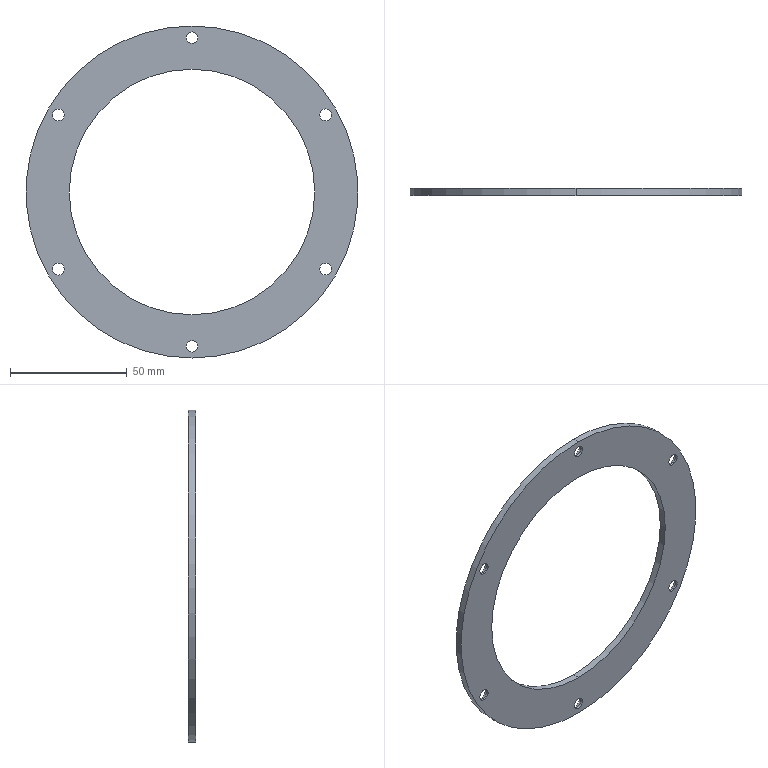Part | SolidWorks | features BaseBody 1 | 1 solid | 36 faces | box 142 x 3 x 142 mm | volume 20812 mm3 | cylinder 28 | plane 8 | commonest cylinder face diameters 5 x12 8 x12 105 x2 142 x2
STEP:
#1=CARTESIAN_POINT('',(0.,3.,52.5));
#2=VERTEX_POINT('',#1);
#3=CARTESIAN_POINT('',(0.,3.,-52.5));
#4=VERTEX_POINT('',#3);
#5=CARTESIAN_POINT('',(0.,3.,0.));
#6=DIRECTION('',(0.,-1.,0.));
#7=DIRECTION('',(0.,0.,-1.));
#8=AXIS2_PLACEMENT_3D('',#5,#6,#7);
#9=CIRCLE('',#8,52.5);
#10=EDGE_CURVE('',#2,#4,#9,.T.);
#11=ORIENTED_EDGE('',*,*,#10,.F.);
#12=CARTESIAN_POINT('',(0.,0.,52.5));
#13=VERTEX_POINT('',#12);
#14=CARTESIAN_POINT('',(0.,3.,52.5));
#15=DIRECTION('',(0.,-1.,0.));
#16=VECTOR('',#15,1000.);
#17=LINE('',#14,#16);
#18=EDGE_CURVE('',#2,#13,#17,.T.);
#19=ORIENTED_EDGE('',*,*,#18,.T.);
#20=CARTESIAN_POINT('',(0.,0.,-52.5));
#21=VERTEX_POINT('',#20);
#22=CARTESIAN_POINT('',(0.,0.,0.));
#23=DIRECTION('',(0.,-1.,0.));
#24=DIRECTION('',(0.,0.,-1.));
#25=AXIS2_PLACEMENT_3D('',#22,#23,#24);
#26=CIRCLE('',#25,52.5);
#27=EDGE_CURVE('',#13,#21,#26,.T.);
#28=ORIENTED_EDGE('',*,*,#27,.T.);
#29=CARTESIAN_POINT('',(0.,3.,-52.5));
#30=DIRECTION('',(0.,-1.,0.));
#31=VECTOR('',#30,1000.);
#32=LINE('',#29,#31);
#33=EDGE_CURVE('',#4,#21,#32,.T.);
#34=ORIENTED_EDGE('',*,*,#33,.F.);
#35=EDGE_LOOP('',(#11,#19,#28,#34));
#36=FACE_OUTER_BOUND('',#35,.T.);
#37=CARTESIAN_POINT('',(0.,3.,0.));
#38=DIRECTION('',(0.,-1.,0.));
#39=DIRECTION('',(0.,0.,-1.));
#40=AXIS2_PLACEMENT_3D('',#37,#38,#39);
#41=CYLINDRICAL_SURFACE('',#40,52.5);
#42=ADVANCED_FACE('',(#36),#41,.F.);
#43=CARTESIAN_POINT('',(0.,3.,-71.));
#44=VERTEX_POINT('',#43);
#45=CARTESIAN_POINT('',(0.,3.,71.));
#46=VERTEX_POINT('',#45);
#47=CARTESIAN_POINT('',(0.,3.,0.));
#48=DIRECTION('',(0.,-1.,0.));
#49=DIRECTION('',(0.,0.,-1.));
#50=AXIS2_PLACEMENT_3D('',#47,#48,#49);
#51=CIRCLE('',#50,71.);
#52=EDGE_CURVE('',#44,#46,#51,.T.);
#53=ORIENTED_EDGE('',*,*,#52,.T.);
#54=CARTESIAN_POINT('',(0.,0.,71.));
#55=VERTEX_POINT('',#54);
#56=CARTESIAN_POINT('',(0.,3.,71.));
#57=DIRECTION('',(0.,-1.,0.));
#58=VECTOR('',#57,1000.);
#59=LINE('',#56,#58);
#60=EDGE_CURVE('',#46,#55,#59,.T.);
#61=ORIENTED_EDGE('',*,*,#60,.T.);
#62=CARTESIAN_POINT('',(0.,0.,-71.));
#63=VERTEX_POINT('',#62);
#64=CARTESIAN_POINT('',(0.,0.,0.));
#65=DIRECTION('',(0.,1.,0.));
#66=DIRECTION('',(0.,0.,-1.));
#67=AXIS2_PLACEMENT_3D('',#64,#65,#66);
#68=CIRCLE('',#67,71.);
#69=EDGE_CURVE('',#55,#63,#68,.T.);
#70=ORIENTED_EDGE('',*,*,#69,.T.);
#71=CARTESIAN_POINT('',(0.,3.,-71.));
#72=DIRECTION('',(0.,-1.,0.));
#73=VECTOR('',#72,1000.);
#74=LINE('',#71,#73);
#75=EDGE_CURVE('',#44,#63,#74,.T.);
#76=ORIENTED_EDGE('',*,*,#75,.F.);
#77=EDGE_LOOP('',(#53,#61,#70,#76));
#78=FACE_OUTER_BOUND('',#77,.T.);
#79=CARTESIAN_POINT('',(0.,3.,0.));
#80=DIRECTION('',(0.,-1.,0.));
#81=DIRECTION('',(0.,0.,-1.));
#82=AXIS2_PLACEMENT_3D('',#79,#80,#81);
#83=CYLINDRICAL_SURFACE('',#82,71.);
#84=ADVANCED_FACE('',(#78),#83,.T.);
#85=CARTESIAN_POINT('',(0.,1.,68.5));
#86=VERTEX_POINT('',#85);
#87=CARTESIAN_POINT('',(0.,1.,63.5));
#88=VERTEX_POINT('',#87);
#89=CARTESIAN_POINT('',(0.,1.,66.));
#90=DIRECTION('',(0.,-1.,0.));
#91=DIRECTION('',(0.,0.,-1.));
#92=AXIS2_PLACEMENT_3D('',#89,#90,#91);
#93=CIRCLE('',#92,2.5);
#94=EDGE_CURVE('',#86,#88,#93,.T.);
#95=ORIENTED_EDGE('',*,*,#94,.F.);
#96=CARTESIAN_POINT('',(0.,0.,68.5));
#97=VERTEX_POINT('',#96);
#98=CARTESIAN_POINT('',(0.,3.,68.5));
#99=DIRECTION('',(0.,-1.,0.));
#100=VECTOR('',#99,1000.);
#101=LINE('',#98,#100);
#102=EDGE_CURVE('',#86,#97,#101,.T.);
#103=ORIENTED_EDGE('',*,*,#102,.T.);
#104=CARTESIAN_POINT('',(0.,0.,63.5));
#105=VERTEX_POINT('',#104);
#106=CARTESIAN_POINT('',(0.,0.,66.));
#107=DIRECTION('',(0.,-1.,0.));
#108=DIRECTION('',(0.,0.,-1.));
#109=AXIS2_PLACEMENT_3D('',#106,#107,#108);
#110=CIRCLE('',#109,2.5);
#111=EDGE_CURVE('',#97,#105,#110,.T.);
#112=ORIENTED_EDGE('',*,*,#111,.T.);
#113=CARTESIAN_POINT('',(0.,3.,63.5));
#114=DIRECTION('',(0.,-1.,0.));
#115=VECTOR('',#114,1000.);
#116=LINE('',#113,#115);
#117=EDGE_CURVE('',#88,#105,#116,.T.);
#118=ORIENTED_EDGE('',*,*,#117,.F.);
#119=EDGE_LOOP('',(#95,#103,#112,#118));
#120=FACE_OUTER_BOUND('',#119,.T.);
#121=CARTESIAN_POINT('',(0.,3.,66.));
#122=DIRECTION('',(0.,-1.,0.));
#123=DIRECTION('',(0.,0.,-1.));
#124=AXIS2_PLACEMENT_3D('',#121,#122,#123);
#125=CYLINDRICAL_SURFACE('',#124,2.5);
#126=ADVANCED_FACE('',(#120),#125,.F.);
#127=CARTESIAN_POINT('',(-57.158,1.,35.5));
#128=VERTEX_POINT('',#127);
#129=CARTESIAN_POINT('',(-57.158,1.,30.5));
#130=VERTEX_POINT('',#129);
#131=CARTESIAN_POINT('',(-57.158,1.,33.));
#132=DIRECTION('',(0.,-1.,0.));
#133=DIRECTION('',(0.,0.,-1.));
#134=AXIS2_PLACEMENT_3D('',#131,#132,#133);
#135=CIRCLE('',#134,2.5);
#136=EDGE_CURVE('',#128,#130,#135,.T.);
#137=ORIENTED_EDGE('',*,*,#136,.F.);
#138=CARTESIAN_POINT('',(-57.158,0.,35.5));
#139=VERTEX_POINT('',#138);
#140=CARTESIAN_POINT('',(-57.158,3.,35.5));
#141=DIRECTION('',(0.,-1.,0.));
#142=VECTOR('',#141,1000.);
#143=LINE('',#140,#142);
#144=EDGE_CURVE('',#128,#139,#143,.T.);
#145=ORIENTED_EDGE('',*,*,#144,.T.);
#146=CARTESIAN_POINT('',(-57.158,0.,30.5));
#147=VERTEX_POINT('',#146);
#148=CARTESIAN_POINT('',(-57.158,0.,33.));
#149=DIRECTION('',(0.,-1.,0.));
#150=DIRECTION('',(0.,0.,-1.));
#151=AXIS2_PLACEMENT_3D('',#148,#149,#150);
#152=CIRCLE('',#151,2.5);
#153=EDGE_CURVE('',#139,#147,#152,.T.);
#154=ORIENTED_EDGE('',*,*,#153,.T.);
#155=CARTESIAN_POINT('',(-57.158,3.,30.5));
#156=DIRECTION('',(0.,-1.,0.));
#157=VECTOR('',#156,1000.);
#158=LINE('',#155,#157);
#159=EDGE_CURVE('',#130,#147,#158,.T.);
#160=ORIENTED_EDGE('',*,*,#159,.F.);
#161=EDGE_LOOP('',(#137,#145,#154,#160));
#162=FACE_OUTER_BOUND('',#161,.T.);
#163=CARTESIAN_POINT('',(-57.158,3.,33.));
#164=DIRECTION('',(0.,-1.,0.));
#165=DIRECTION('',(0.,0.,-1.));
#166=AXIS2_PLACEMENT_3D('',#163,#164,#165);
#167=CYLINDRICAL_SURFACE('',#166,2.5);
#168=ADVANCED_FACE('',(#162),#167,.F.);
#169=CARTESIAN_POINT('',(-57.158,1.,-30.5));
#170=VERTEX_POINT('',#169);
#171=CARTESIAN_POINT('',(-57.158,1.,-35.5));
#172=VERTEX_POINT('',#171);
#173=CARTESIAN_POINT('',(-57.158,1.,-33.));
#174=DIRECTION('',(0.,-1.,0.));
#175=DIRECTION('',(0.,0.,-1.));
#176=AXIS2_PLACEMENT_3D('',#173,#174,#175);
#177=CIRCLE('',#176,2.5);
#178=EDGE_CURVE('',#170,#172,#177,.T.);
#179=ORIENTED_EDGE('',*,*,#178,.F.);
#180=CARTESIAN_POINT('',(-57.158,0.,-30.5));
#181=VERTEX_POINT('',#180);
#182=CARTESIAN_POINT('',(-57.158,3.,-30.5));
#183=DIRECTION('',(0.,-1.,0.));
#184=VECTOR('',#183,1000.);
#185=LINE('',#182,#184);
#186=EDGE_CURVE('',#170,#181,#185,.T.);
#187=ORIENTED_EDGE('',*,*,#186,.T.);
#188=CARTESIAN_POINT('',(-57.158,0.,-35.5));
#189=VERTEX_POINT('',#188);
#190=CARTESIAN_POINT('',(-57.158,0.,-33.));
#191=DIRECTION('',(0.,-1.,0.));
#192=DIRECTION('',(0.,0.,-1.));
#193=AXIS2_PLACEMENT_3D('',#190,#191,#192);
#194=CIRCLE('',#193,2.5);
#195=EDGE_CURVE('',#181,#189,#194,.T.);
#196=ORIENTED_EDGE('',*,*,#195,.T.);
#197=CARTESIAN_POINT('',(-57.158,3.,-35.5));
#198=DIRECTION('',(0.,-1.,0.));
#199=VECTOR('',#198,1000.);
#200=LINE('',#197,#199);
#201=EDGE_CURVE('',#172,#189,#200,.T.);
#202=ORIENTED_EDGE('',*,*,#201,.F.);
#203=EDGE_LOOP('',(#179,#187,#196,#202));
#204=FACE_OUTER_BOUND('',#203,.T.);
#205=CARTESIAN_POINT('',(-57.158,3.,-33.));
#206=DIRECTION('',(0.,-1.,0.));
#207=DIRECTION('',(0.,0.,-1.));
#208=AXIS2_PLACEMENT_3D('',#205,#206,#207);
#209=CYLINDRICAL_SURFACE('',#208,2.5);
#210=ADVANCED_FACE('',(#204),#209,.F.);
#211=CARTESIAN_POINT('',(0.,1.,-63.5));
#212=VERTEX_POINT('',#211);
#213=CARTESIAN_POINT('',(0.,1.,-68.5));
#214=VERTEX_POINT('',#213);
#215=CARTESIAN_POINT('',(0.,1.,-66.));
#216=DIRECTION('',(0.,-1.,0.));
#217=DIRECTION('',(0.,0.,-1.));
#218=AXIS2_PLACEMENT_3D('',#215,#216,#217);
#219=CIRCLE('',#218,2.5);
#220=EDGE_CURVE('',#212,#214,#219,.T.);
#221=ORIENTED_EDGE('',*,*,#220,.F.);
#222=CARTESIAN_POINT('',(0.,0.,-63.5));
#223=VERTEX_POINT('',#222);
#224=CARTESIAN_POINT('',(0.,3.,-63.5));
#225=DIRECTION('',(0.,-1.,0.));
#226=VECTOR('',#225,1000.);
#227=LINE('',#224,#226);
#228=EDGE_CURVE('',#212,#223,#227,.T.);
#229=ORIENTED_EDGE('',*,*,#228,.T.);
#230=CARTESIAN_POINT('',(0.,0.,-68.5));
#231=VERTEX_POINT('',#230);
#232=CARTESIAN_POINT('',(0.,0.,-66.));
#233=DIRECTION('',(0.,-1.,0.));
#234=DIRECTION('',(0.,0.,-1.));
#235=AXIS2_PLACEMENT_3D('',#232,#233,#234);
#236=CIRCLE('',#235,2.5);
#237=EDGE_CURVE('',#223,#231,#236,.T.);
#238=ORIENTED_EDGE('',*,*,#237,.T.);
#239=CARTESIAN_POINT('',(0.,3.,-68.5));
#240=DIRECTION('',(0.,-1.,0.));
#241=VECTOR('',#240,1000.);
#242=LINE('',#239,#241);
#243=EDGE_CURVE('',#214,#231,#242,.T.);
#244=ORIENTED_EDGE('',*,*,#243,.F.);
#245=EDGE_LOOP('',(#221,#229,#238,#244));
#246=FACE_OUTER_BOUND('',#245,.T.);
#247=CARTESIAN_POINT('',(0.,3.,-66.));
#248=DIRECTION('',(0.,-1.,0.));
#249=DIRECTION('',(0.,0.,-1.));
#250=AXIS2_PLACEMENT_3D('',#247,#248,#249);
#251=CYLINDRICAL_SURFACE('',#250,2.5);
#252=ADVANCED_FACE('',(#246),#251,.F.);
#253=CARTESIAN_POINT('',(57.158,1.,-30.5));
#254=VERTEX_POINT('',#253);
#255=CARTESIAN_POINT('',(57.158,1.,-35.5));
#256=VERTEX_POINT('',#255);
#257=CARTESIAN_POINT('',(57.158,1.,-33.));
#258=DIRECTION('',(0.,-1.,0.));
#259=DIRECTION('',(0.,0.,-1.));
#260=AXIS2_PLACEMENT_3D('',#257,#258,#259);
#261=CIRCLE('',#260,2.5);
#262=EDGE_CURVE('',#254,#256,#261,.T.);
#263=ORIENTED_EDGE('',*,*,#262,.F.);
#264=CARTESIAN_POINT('',(57.158,0.,-30.5));
#265=VERTEX_POINT('',#264);
#266=CARTESIAN_POINT('',(57.158,3.,-30.5));
#267=DIRECTION('',(0.,-1.,0.));
#268=VECTOR('',#267,1000.);
#269=LINE('',#266,#268);
#270=EDGE_CURVE('',#254,#265,#269,.T.);
#271=ORIENTED_EDGE('',*,*,#270,.T.);
#272=CARTESIAN_POINT('',(57.158,0.,-35.5));
#273=VERTEX_POINT('',#272);
#274=CARTESIAN_POINT('',(57.158,0.,-33.));
#275=DIRECTION('',(0.,-1.,0.));
#276=DIRECTION('',(0.,0.,-1.));
#277=AXIS2_PLACEMENT_3D('',#274,#275,#276);
#278=CIRCLE('',#277,2.5);
#279=EDGE_CURVE('',#265,#273,#278,.T.);
#280=ORIENTED_EDGE('',*,*,#279,.T.);
#281=CARTESIAN_POINT('',(57.158,3.,-35.5));
#282=DIRECTION('',(0.,-1.,0.));
#283=VECTOR('',#282,1000.);
#284=LINE('',#281,#283);
#285=EDGE_CURVE('',#256,#273,#284,.T.);
#286=ORIENTED_EDGE('',*,*,#285,.F.);
#287=EDGE_LOOP('',(#263,#271,#280,#286));
#288=FACE_OUTER_BOUND('',#287,.T.);
#289=CARTESIAN_POINT('',(57.158,3.,-33.));
#290=DIRECTION('',(0.,-1.,0.));
#291=DIRECTION('',(0.,0.,-1.));
#292=AXIS2_PLACEMENT_3D('',#289,#290,#291);
#293=CYLINDRICAL_SURFACE('',#292,2.5);
#294=ADVANCED_FACE('',(#288),#293,.F.);
#295=CARTESIAN_POINT('',(57.158,1.,35.5));
#296=VERTEX_POINT('',#295);
#297=CARTESIAN_POINT('',(57.158,1.,30.5));
#298=VERTEX_POINT('',#297);
#299=CARTESIAN_POINT('',(57.158,1.,33.));
#300=DIRECTION('',(0.,-1.,0.));
#301=DIRECTION('',(0.,0.,-1.));
#302=AXIS2_PLACEMENT_3D('',#299,#300,#301);
#303=CIRCLE('',#302,2.5);
#304=EDGE_CURVE('',#296,#298,#303,.T.);
#305=ORIENTED_EDGE('',*,*,#304,.F.);
#306=CARTESIAN_POINT('',(57.158,0.,35.5));
#307=VERTEX_POINT('',#306);
#308=CARTESIAN_POINT('',(57.158,3.,35.5));
#309=DIRECTION('',(0.,-1.,0.));
#310=VECTOR('',#309,1000.);
#311=LINE('',#308,#310);
#312=EDGE_CURVE('',#296,#307,#311,.T.);
#313=ORIENTED_EDGE('',*,*,#312,.T.);
#314=CARTESIAN_POINT('',(57.158,0.,30.5));
#315=VERTEX_POINT('',#314);
#316=CARTESIAN_POINT('',(57.158,0.,33.));
#317=DIRECTION('',(0.,-1.,0.));
#318=DIRECTION('',(0.,0.,-1.));
#319=AXIS2_PLACEMENT_3D('',#316,#317,#318);
#320=CIRCLE('',#319,2.5);
#321=EDGE_CURVE('',#307,#315,#320,.T.);
#322=ORIENTED_EDGE('',*,*,#321,.T.);
#323=CARTESIAN_POINT('',(57.158,3.,30.5));
#324=DIRECTION('',(0.,-1.,0.));
#325=VECTOR('',#324,1000.);
#326=LINE('',#323,#325);
#327=EDGE_CURVE('',#298,#315,#326,.T.);
#328=ORIENTED_EDGE('',*,*,#327,.F.);
#329=EDGE_LOOP('',(#305,#313,#322,#328));
#330=FACE_OUTER_BOUND('',#329,.T.);
#331=CARTESIAN_POINT('',(57.158,3.,33.));
#332=DIRECTION('',(0.,-1.,0.));
#333=DIRECTION('',(0.,0.,-1.));
#334=AXIS2_PLACEMENT_3D('',#331,#332,#333);
#335=CYLINDRICAL_SURFACE('',#334,2.5);
#336=ADVANCED_FACE('',(#330),#335,.F.);
#337=CARTESIAN_POINT('',(0.,1.,-70.));
#338=VERTEX_POINT('',#337);
#339=CARTESIAN_POINT('',(0.,1.,-62.));
#340=VERTEX_POINT('',#339);
#341=CARTESIAN_POINT('',(0.,1.,-66.));
#342=DIRECTION('',(0.,1.,0.));
#343=DIRECTION('',(0.,0.,1.));
#344=AXIS2_PLACEMENT_3D('',#341,#342,#343);
#345=CIRCLE('',#344,4.);
#346=EDGE_CURVE('',#338,#340,#345,.T.);
#347=ORIENTED_EDGE('',*,*,#346,.F.);
#348=CARTESIAN_POINT('',(0.,3.,-70.));
#349=VERTEX_POINT('',#348);
#350=CARTESIAN_POINT('',(0.,1.,-70.));
#351=DIRECTION('',(0.,1.,0.));
#352=VECTOR('',#351,1000.);
#353=LINE('',#350,#352);
#354=EDGE_CURVE('',#338,#349,#353,.T.);
#355=ORIENTED_EDGE('',*,*,#354,.T.);
#356=CARTESIAN_POINT('',(0.,3.,-62.));
#357=VERTEX_POINT('',#356);
#358=CARTESIAN_POINT('',(0.,3.,-66.));
#359=DIRECTION('',(0.,-1.,0.));
#360=DIRECTION('',(0.,0.,1.));
#361=AXIS2_PLACEMENT_3D('',#358,#359,#360);
#362=CIRCLE('',#361,4.);
#363=EDGE_CURVE('',#357,#349,#362,.T.);
#364=ORIENTED_EDGE('',*,*,#363,.F.);
#365=CARTESIAN_POINT('',(0.,1.,-62.));
#366=DIRECTION('',(0.,1.,0.));
#367=VECTOR('',#366,1000.);
#368=LINE('',#365,#367);
#369=EDGE_CURVE('',#340,#357,#368,.T.);
#370=ORIENTED_EDGE('',*,*,#369,.F.);
#371=EDGE_LOOP('',(#347,#355,#364,#370));
#372=FACE_OUTER_BOUND('',#371,.T.);
#373=CARTESIAN_POINT('',(0.,1.,-66.));
#374=DIRECTION('',(0.,1.,0.));
#375=DIRECTION('',(0.,0.,1.));
#376=AXIS2_PLACEMENT_3D('',#373,#374,#375);
#377=CYLINDRICAL_SURFACE('',#376,4.);
#378=ADVANCED_FACE('',(#372),#377,.F.);
#379=CARTESIAN_POINT('',(57.158,1.,-37.));
#380=VERTEX_POINT('',#379);
#381=CARTESIAN_POINT('',(57.158,1.,-29.));
#382=VERTEX_POINT('',#381);
#383=CARTESIAN_POINT('',(57.158,1.,-33.));
#384=DIRECTION('',(0.,1.,0.));
#385=DIRECTION('',(0.,0.,1.));
#386=AXIS2_PLACEMENT_3D('',#383,#384,#385);
#387=CIRCLE('',#386,4.);
#388=EDGE_CURVE('',#380,#382,#387,.T.);
#389=ORIENTED_EDGE('',*,*,#388,.F.);
#390=CARTESIAN_POINT('',(57.158,3.,-37.));
#391=VERTEX_POINT('',#390);
#392=CARTESIAN_POINT('',(57.158,1.,-37.));
#393=DIRECTION('',(0.,1.,0.));
#394=VECTOR('',#393,1000.);
#395=LINE('',#392,#394);
#396=EDGE_CURVE('',#380,#391,#395,.T.);
#397=ORIENTED_EDGE('',*,*,#396,.T.);
#398=CARTESIAN_POINT('',(57.158,3.,-29.));
#399=VERTEX_POINT('',#398);
#400=CARTESIAN_POINT('',(57.158,3.,-33.));
#401=DIRECTION('',(0.,-1.,0.));
#402=DIRECTION('',(0.,0.,1.));
#403=AXIS2_PLACEMENT_3D('',#400,#401,#402);
#404=CIRCLE('',#403,4.);
#405=EDGE_CURVE('',#399,#391,#404,.T.);
#406=ORIENTED_EDGE('',*,*,#405,.F.);
#407=CARTESIAN_POINT('',(57.158,1.,-29.));
#408=DIRECTION('',(0.,1.,0.));
#409=VECTOR('',#408,1000.);
#410=LINE('',#407,#409);
#411=EDGE_CURVE('',#382,#399,#410,.T.);
#412=ORIENTED_EDGE('',*,*,#411,.F.);
#413=EDGE_LOOP('',(#389,#397,#406,#412));
#414=FACE_OUTER_BOUND('',#413,.T.);
#415=CARTESIAN_POINT('',(57.158,1.,-33.));
#416=DIRECTION('',(0.,1.,0.));
#417=DIRECTION('',(0.,0.,1.));
#418=AXIS2_PLACEMENT_3D('',#415,#416,#417);
#419=CYLINDRICAL_SURFACE('',#418,4.);
#420=ADVANCED_FACE('',(#414),#419,.F.);
#421=CARTESIAN_POINT('',(57.158,1.,29.));
#422=VERTEX_POINT('',#421);
#423=CARTESIAN_POINT('',(57.158,1.,37.));
#424=VERTEX_POINT('',#423);
#425=CARTESIAN_POINT('',(57.158,1.,33.));
#426=DIRECTION('',(0.,1.,0.));
#427=DIRECTION('',(0.,0.,1.));
#428=AXIS2_PLACEMENT_3D('',#425,#426,#427);
#429=CIRCLE('',#428,4.);
#430=EDGE_CURVE('',#422,#424,#429,.T.);
#431=ORIENTED_EDGE('',*,*,#430,.F.);
#432=CARTESIAN_POINT('',(57.158,3.,29.));
#433=VERTEX_POINT('',#432);
#434=CARTESIAN_POINT('',(57.158,1.,29.));
#435=DIRECTION('',(0.,1.,0.));
#436=VECTOR('',#435,1000.);
#437=LINE('',#434,#436);
#438=EDGE_CURVE('',#422,#433,#437,.T.);
#439=ORIENTED_EDGE('',*,*,#438,.T.);
#440=CARTESIAN_POINT('',(57.158,3.,37.));
#441=VERTEX_POINT('',#440);
#442=CARTESIAN_POINT('',(57.158,3.,33.));
#443=DIRECTION('',(0.,-1.,0.));
#444=DIRECTION('',(0.,0.,1.));
#445=AXIS2_PLACEMENT_3D('',#442,#443,#444);
#446=CIRCLE('',#445,4.);
#447=EDGE_CURVE('',#441,#433,#446,.T.);
#448=ORIENTED_EDGE('',*,*,#447,.F.);
#449=CARTESIAN_POINT('',(57.158,1.,37.));
#450=DIRECTION('',(0.,1.,0.));
#451=VECTOR('',#450,1000.);
#452=LINE('',#449,#451);
#453=EDGE_CURVE('',#424,#441,#452,.T.);
#454=ORIENTED_EDGE('',*,*,#453,.F.);
#455=EDGE_LOOP('',(#431,#439,#448,#454));
#456=FACE_OUTER_BOUND('',#455,.T.);
#457=CARTESIAN_POINT('',(57.158,1.,33.));
#458=DIRECTION('',(0.,1.,0.));
#459=DIRECTION('',(0.,0.,1.));
#460=AXIS2_PLACEMENT_3D('',#457,#458,#459);
#461=CYLINDRICAL_SURFACE('',#460,4.);
#462=ADVANCED_FACE('',(#456),#461,.F.);
#463=CARTESIAN_POINT('',(0.,1.,62.));
#464=VERTEX_POINT('',#463);
#465=CARTESIAN_POINT('',(0.,1.,70.));
#466=VERTEX_POINT('',#465);
#467=CARTESIAN_POINT('',(0.,1.,66.));
#468=DIRECTION('',(0.,1.,0.));
#469=DIRECTION('',(0.,0.,1.));
#470=AXIS2_PLACEMENT_3D('',#467,#468,#469);
#471=CIRCLE('',#470,4.);
#472=EDGE_CURVE('',#464,#466,#471,.T.);
#473=ORIENTED_EDGE('',*,*,#472,.F.);
#474=CARTESIAN_POINT('',(0.,3.,62.));
#475=VERTEX_POINT('',#474);
#476=CARTESIAN_POINT('',(0.,1.,62.));
#477=DIRECTION('',(0.,1.,0.));
#478=VECTOR('',#477,1000.);
#479=LINE('',#476,#478);
#480=EDGE_CURVE('',#464,#475,#479,.T.);
#481=ORIENTED_EDGE('',*,*,#480,.T.);
#482=CARTESIAN_POINT('',(0.,3.,70.));
#483=VERTEX_POINT('',#482);
#484=CARTESIAN_POINT('',(0.,3.,66.));
#485=DIRECTION('',(0.,-1.,0.));
#486=DIRECTION('',(0.,0.,1.));
#487=AXIS2_PLACEMENT_3D('',#484,#485,#486);
#488=CIRCLE('',#487,4.);
#489=EDGE_CURVE('',#483,#475,#488,.T.);
#490=ORIENTED_EDGE('',*,*,#489,.F.);
#491=CARTESIAN_POINT('',(0.,1.,70.));
#492=DIRECTION('',(0.,1.,0.));
#493=VECTOR('',#492,1000.);
#494=LINE('',#491,#493);
#495=EDGE_CURVE('',#466,#483,#494,.T.);
#496=ORIENTED_EDGE('',*,*,#495,.F.);
#497=EDGE_LOOP('',(#473,#481,#490,#496));
#498=FACE_OUTER_BOUND('',#497,.T.);
#499=CARTESIAN_POINT('',(0.,1.,66.));
#500=DIRECTION('',(0.,1.,0.));
#501=DIRECTION('',(0.,0.,1.));
#502=AXIS2_PLACEMENT_3D('',#499,#500,#501);
#503=CYLINDRICAL_SURFACE('',#502,4.);
#504=ADVANCED_FACE('',(#498),#503,.F.);
#505=CARTESIAN_POINT('',(-57.158,1.,29.));
#506=VERTEX_POINT('',#505);
#507=CARTESIAN_POINT('',(-57.158,1.,37.));
#508=VERTEX_POINT('',#507);
#509=CARTESIAN_POINT('',(-57.158,1.,33.));
#510=DIRECTION('',(0.,1.,0.));
#511=DIRECTION('',(0.,0.,1.));
#512=AXIS2_PLACEMENT_3D('',#509,#510,#511);
#513=CIRCLE('',#512,4.);
#514=EDGE_CURVE('',#506,#508,#513,.T.);
#515=ORIENTED_EDGE('',*,*,#514,.F.);
#516=CARTESIAN_POINT('',(-57.158,3.,29.));
#517=VERTEX_POINT('',#516);
#518=CARTESIAN_POINT('',(-57.158,1.,29.));
#519=DIRECTION('',(0.,1.,0.));
#520=VECTOR('',#519,1000.);
#521=LINE('',#518,#520);
#522=EDGE_CURVE('',#506,#517,#521,.T.);
#523=ORIENTED_EDGE('',*,*,#522,.T.);
#524=CARTESIAN_POINT('',(-57.158,3.,37.));
#525=VERTEX_POINT('',#524);
#526=CARTESIAN_POINT('',(-57.158,3.,33.));
#527=DIRECTION('',(0.,-1.,0.));
#528=DIRECTION('',(0.,0.,1.));
#529=AXIS2_PLACEMENT_3D('',#526,#527,#528);
#530=CIRCLE('',#529,4.);
#531=EDGE_CURVE('',#525,#517,#530,.T.);
#532=ORIENTED_EDGE('',*,*,#531,.F.);
#533=CARTESIAN_POINT('',(-57.158,1.,37.));
#534=DIRECTION('',(0.,1.,0.));
#535=VECTOR('',#534,1000.);
#536=LINE('',#533,#535);
#537=EDGE_CURVE('',#508,#525,#536,.T.);
#538=ORIENTED_EDGE('',*,*,#537,.F.);
#539=EDGE_LOOP('',(#515,#523,#532,#538));
#540=FACE_OUTER_BOUND('',#539,.T.);
#541=CARTESIAN_POINT('',(-57.158,1.,33.));
#542=DIRECTION('',(0.,1.,0.));
#543=DIRECTION('',(0.,0.,1.));
#544=AXIS2_PLACEMENT_3D('',#541,#542,#543);
#545=CYLINDRICAL_SURFACE('',#544,4.);
#546=ADVANCED_FACE('',(#540),#545,.F.);
#547=CARTESIAN_POINT('',(-57.158,1.,-37.));
#548=VERTEX_POINT('',#547);
#549=CARTESIAN_POINT('',(-57.158,1.,-29.));
#550=VERTEX_POINT('',#549);
#551=CARTESIAN_POINT('',(-57.158,1.,-33.));
#552=DIRECTION('',(0.,1.,0.));
#553=DIRECTION('',(0.,0.,1.));
#554=AXIS2_PLACEMENT_3D('',#551,#552,#553);
#555=CIRCLE('',#554,4.);
#556=EDGE_CURVE('',#548,#550,#555,.T.);
#557=ORIENTED_EDGE('',*,*,#556,.F.);
#558=CARTESIAN_POINT('',(-57.158,3.,-37.));
#559=VERTEX_POINT('',#558);
#560=CARTESIAN_POINT('',(-57.158,1.,-37.));
#561=DIRECTION('',(0.,1.,0.));
#562=VECTOR('',#561,1000.);
#563=LINE('',#560,#562);
#564=EDGE_CURVE('',#548,#559,#563,.T.);
#565=ORIENTED_EDGE('',*,*,#564,.T.);
#566=CARTESIAN_POINT('',(-57.158,3.,-29.));
#567=VERTEX_POINT('',#566);
#568=CARTESIAN_POINT('',(-57.158,3.,-33.));
#569=DIRECTION('',(0.,-1.,0.));
#570=DIRECTION('',(0.,0.,1.));
#571=AXIS2_PLACEMENT_3D('',#568,#569,#570);
#572=CIRCLE('',#571,4.);
#573=EDGE_CURVE('',#567,#559,#572,.T.);
#574=ORIENTED_EDGE('',*,*,#573,.F.);
#575=CARTESIAN_POINT('',(-57.158,1.,-29.));
#576=DIRECTION('',(0.,1.,0.));
#577=VECTOR('',#576,1000.);
#578=LINE('',#575,#577);
#579=EDGE_CURVE('',#550,#567,#578,.T.);
#580=ORIENTED_EDGE('',*,*,#579,.F.);
#581=EDGE_LOOP('',(#557,#565,#574,#580));
#582=FACE_OUTER_BOUND('',#581,.T.);
#583=CARTESIAN_POINT('',(-57.158,1.,-33.));
#584=DIRECTION('',(0.,1.,0.));
#585=DIRECTION('',(0.,0.,1.));
#586=AXIS2_PLACEMENT_3D('',#583,#584,#585);
#587=CYLINDRICAL_SURFACE('',#586,4.);
#588=ADVANCED_FACE('',(#582),#587,.F.);
#589=CARTESIAN_POINT('',(0.,0.,0.));
#590=DIRECTION('',(0.,-1.,0.));
#591=DIRECTION('',(0.,0.,-1.));
#592=AXIS2_PLACEMENT_3D('',#589,#590,#591);
#593=CIRCLE('',#592,52.5);
#594=EDGE_CURVE('',#21,#13,#593,.T.);
#595=ORIENTED_EDGE('',*,*,#594,.F.);
#596=ORIENTED_EDGE('',*,*,#27,.F.);
#597=EDGE_LOOP('',(#595,#596));
#598=FACE_BOUND('',#597,.T.);
#599=CARTESIAN_POINT('',(0.,0.,0.));
#600=DIRECTION('',(0.,1.,0.));
#601=DIRECTION('',(0.,0.,-1.));
#602=AXIS2_PLACEMENT_3D('',#599,#600,#601);
#603=CIRCLE('',#602,71.);
#604=EDGE_CURVE('',#63,#55,#603,.T.);
#605=ORIENTED_EDGE('',*,*,#604,.F.);
#606=ORIENTED_EDGE('',*,*,#69,.F.);
#607=EDGE_LOOP('',(#605,#606));
#608=FACE_OUTER_BOUND('',#607,.T.);
#609=CARTESIAN_POINT('',(0.,0.,66.));
#610=DIRECTION('',(0.,-1.,0.));
#611=DIRECTION('',(0.,0.,-1.));
#612=AXIS2_PLACEMENT_3D('',#609,#610,#611);
#613=CIRCLE('',#612,2.5);
#614=EDGE_CURVE('',#105,#97,#613,.T.);
#615=ORIENTED_EDGE('',*,*,#614,.F.);
#616=ORIENTED_EDGE('',*,*,#111,.F.);
#617=EDGE_LOOP('',(#615,#616));
#618=FACE_BOUND('',#617,.T.);
#619=CARTESIAN_POINT('',(-57.158,0.,33.));
#620=DIRECTION('',(0.,-1.,0.));
#621=DIRECTION('',(0.,0.,-1.));
#622=AXIS2_PLACEMENT_3D('',#619,#620,#621);
#623=CIRCLE('',#622,2.5);
#624=EDGE_CURVE('',#147,#139,#623,.T.);
#625=ORIENTED_EDGE('',*,*,#624,.F.);
#626=ORIENTED_EDGE('',*,*,#153,.F.);
#627=EDGE_LOOP('',(#625,#626));
#628=FACE_BOUND('',#627,.T.);
#629=CARTESIAN_POINT('',(-57.158,0.,-33.));
#630=DIRECTION('',(0.,-1.,0.));
#631=DIRECTION('',(0.,0.,-1.));
#632=AXIS2_PLACEMENT_3D('',#629,#630,#631);
#633=CIRCLE('',#632,2.5);
#634=EDGE_CURVE('',#189,#181,#633,.T.);
#635=ORIENTED_EDGE('',*,*,#634,.F.);
#636=ORIENTED_EDGE('',*,*,#195,.F.);
#637=EDGE_LOOP('',(#635,#636));
#638=FACE_BOUND('',#637,.T.);
#639=CARTESIAN_POINT('',(0.,0.,-66.));
#640=DIRECTION('',(0.,-1.,0.));
#641=DIRECTION('',(0.,0.,-1.));
#642=AXIS2_PLACEMENT_3D('',#639,#640,#641);
#643=CIRCLE('',#642,2.5);
#644=EDGE_CURVE('',#231,#223,#643,.T.);
#645=ORIENTED_EDGE('',*,*,#644,.F.);
#646=ORIENTED_EDGE('',*,*,#237,.F.);
#647=EDGE_LOOP('',(#645,#646));
#648=FACE_BOUND('',#647,.T.);
#649=CARTESIAN_POINT('',(57.158,0.,-33.));
#650=DIRECTION('',(0.,-1.,0.));
#651=DIRECTION('',(0.,0.,-1.));
#652=AXIS2_PLACEMENT_3D('',#649,#650,#651);
#653=CIRCLE('',#652,2.5);
#654=EDGE_CURVE('',#273,#265,#653,.T.);
#655=ORIENTED_EDGE('',*,*,#654,.F.);
#656=ORIENTED_EDGE('',*,*,#279,.F.);
#657=EDGE_LOOP('',(#655,#656));
#658=FACE_BOUND('',#657,.T.);
#659=CARTESIAN_POINT('',(57.158,0.,33.));
#660=DIRECTION('',(0.,-1.,0.));
#661=DIRECTION('',(0.,0.,-1.));
#662=AXIS2_PLACEMENT_3D('',#659,#660,#661);
#663=CIRCLE('',#662,2.5);
#664=EDGE_CURVE('',#315,#307,#663,.T.);
#665=ORIENTED_EDGE('',*,*,#664,.F.);
#666=ORIENTED_EDGE('',*,*,#321,.F.);
#667=EDGE_LOOP('',(#665,#666));
#668=FACE_BOUND('',#667,.T.);
#669=CARTESIAN_POINT('',(0.,0.,0.));
#670=DIRECTION('',(0.,1.,0.));
#671=DIRECTION('',(0.,0.,1.));
#672=AXIS2_PLACEMENT_3D('',#669,#670,#671);
#673=PLANE('',#672);
#674=ADVANCED_FACE('',(#598,#608,#618,#628,#638,#648,#658,#668),#673,.F.);
#675=ORIENTED_EDGE('',*,*,#18,.F.);
#676=CARTESIAN_POINT('',(0.,3.,0.));
#677=DIRECTION('',(0.,-1.,0.));
#678=DIRECTION('',(0.,0.,-1.));
#679=AXIS2_PLACEMENT_3D('',#676,#677,#678);
#680=CIRCLE('',#679,52.5);
#681=EDGE_CURVE('',#4,#2,#680,.T.);
#682=ORIENTED_EDGE('',*,*,#681,.F.);
#683=ORIENTED_EDGE('',*,*,#33,.T.);
#684=ORIENTED_EDGE('',*,*,#594,.T.);
#685=EDGE_LOOP('',(#675,#682,#683,#684));
#686=FACE_OUTER_BOUND('',#685,.T.);
#687=CARTESIAN_POINT('',(0.,3.,0.));
#688=DIRECTION('',(0.,-1.,0.));
#689=DIRECTION('',(0.,0.,-1.));
#690=AXIS2_PLACEMENT_3D('',#687,#688,#689);
#691=CYLINDRICAL_SURFACE('',#690,52.5);
#692=ADVANCED_FACE('',(#686),#691,.F.);
#693=ORIENTED_EDGE('',*,*,#60,.F.);
#694=CARTESIAN_POINT('',(0.,3.,0.));
#695=DIRECTION('',(0.,-1.,0.));
#696=DIRECTION('',(0.,0.,-1.));
#697=AXIS2_PLACEMENT_3D('',#694,#695,#696);
#698=CIRCLE('',#697,71.);
#699=EDGE_CURVE('',#46,#44,#698,.T.);
#700=ORIENTED_EDGE('',*,*,#699,.T.);
#701=ORIENTED_EDGE('',*,*,#75,.T.);
#702=ORIENTED_EDGE('',*,*,#604,.T.);
#703=EDGE_LOOP('',(#693,#700,#701,#702));
#704=FACE_OUTER_BOUND('',#703,.T.);
#705=CARTESIAN_POINT('',(0.,3.,0.));
#706=DIRECTION('',(0.,-1.,0.));
#707=DIRECTION('',(0.,0.,-1.));
#708=AXIS2_PLACEMENT_3D('',#705,#706,#707);
#709=CYLINDRICAL_SURFACE('',#708,71.);
#710=ADVANCED_FACE('',(#704),#709,.T.);
#711=ORIENTED_EDGE('',*,*,#102,.F.);
#712=CARTESIAN_POINT('',(0.,1.,66.));
#713=DIRECTION('',(0.,-1.,0.));
#714=DIRECTION('',(0.,0.,-1.));
#715=AXIS2_PLACEMENT_3D('',#712,#713,#714);
#716=CIRCLE('',#715,2.5);
#717=EDGE_CURVE('',#88,#86,#716,.T.);
#718=ORIENTED_EDGE('',*,*,#717,.F.);
#719=ORIENTED_EDGE('',*,*,#117,.T.);
#720=ORIENTED_EDGE('',*,*,#614,.T.);
#721=EDGE_LOOP('',(#711,#718,#719,#720));
#722=FACE_OUTER_BOUND('',#721,.T.);
#723=CARTESIAN_POINT('',(0.,3.,66.));
#724=DIRECTION('',(0.,-1.,0.));
#725=DIRECTION('',(0.,0.,-1.));
#726=AXIS2_PLACEMENT_3D('',#723,#724,#725);
#727=CYLINDRICAL_SURFACE('',#726,2.5);
#728=ADVANCED_FACE('',(#722),#727,.F.);
#729=ORIENTED_EDGE('',*,*,#144,.F.);
#730=CARTESIAN_POINT('',(-57.158,1.,33.));
#731=DIRECTION('',(0.,-1.,0.));
#732=DIRECTION('',(0.,0.,-1.));
#733=AXIS2_PLACEMENT_3D('',#730,#731,#732);
#734=CIRCLE('',#733,2.5);
#735=EDGE_CURVE('',#130,#128,#734,.T.);
#736=ORIENTED_EDGE('',*,*,#735,.F.);
#737=ORIENTED_EDGE('',*,*,#159,.T.);
#738=ORIENTED_EDGE('',*,*,#624,.T.);
#739=EDGE_LOOP('',(#729,#736,#737,#738));
#740=FACE_OUTER_BOUND('',#739,.T.);
#741=CARTESIAN_POINT('',(-57.158,3.,33.));
#742=DIRECTION('',(0.,-1.,0.));
#743=DIRECTION('',(0.,0.,-1.));
#744=AXIS2_PLACEMENT_3D('',#741,#742,#743);
#745=CYLINDRICAL_SURFACE('',#744,2.5);
#746=ADVANCED_FACE('',(#740),#745,.F.);
#747=ORIENTED_EDGE('',*,*,#186,.F.);
#748=CARTESIAN_POINT('',(-57.158,1.,-33.));
#749=DIRECTION('',(0.,-1.,0.));
#750=DIRECTION('',(0.,0.,-1.));
#751=AXIS2_PLACEMENT_3D('',#748,#749,#750);
#752=CIRCLE('',#751,2.5);
#753=EDGE_CURVE('',#172,#170,#752,.T.);
#754=ORIENTED_EDGE('',*,*,#753,.F.);
#755=ORIENTED_EDGE('',*,*,#201,.T.);
#756=ORIENTED_EDGE('',*,*,#634,.T.);
#757=EDGE_LOOP('',(#747,#754,#755,#756));
#758=FACE_OUTER_BOUND('',#757,.T.);
#759=CARTESIAN_POINT('',(-57.158,3.,-33.));
#760=DIRECTION('',(0.,-1.,0.));
#761=DIRECTION('',(0.,0.,-1.));
#762=AXIS2_PLACEMENT_3D('',#759,#760,#761);
#763=CYLINDRICAL_SURFACE('',#762,2.5);
#764=ADVANCED_FACE('',(#758),#763,.F.);
#765=ORIENTED_EDGE('',*,*,#228,.F.);
#766=CARTESIAN_POINT('',(0.,1.,-66.));
#767=DIRECTION('',(0.,-1.,0.));
#768=DIRECTION('',(0.,0.,-1.));
#769=AXIS2_PLACEMENT_3D('',#766,#767,#768);
#770=CIRCLE('',#769,2.5);
#771=EDGE_CURVE('',#214,#212,#770,.T.);
#772=ORIENTED_EDGE('',*,*,#771,.F.);
#773=ORIENTED_EDGE('',*,*,#243,.T.);
#774=ORIENTED_EDGE('',*,*,#644,.T.);
#775=EDGE_LOOP('',(#765,#772,#773,#774));
#776=FACE_OUTER_BOUND('',#775,.T.);
#777=CARTESIAN_POINT('',(0.,3.,-66.));
#778=DIRECTION('',(0.,-1.,0.));
#779=DIRECTION('',(0.,0.,-1.));
#780=AXIS2_PLACEMENT_3D('',#777,#778,#779);
#781=CYLINDRICAL_SURFACE('',#780,2.5);
#782=ADVANCED_FACE('',(#776),#781,.F.);
#783=ORIENTED_EDGE('',*,*,#270,.F.);
#784=CARTESIAN_POINT('',(57.158,1.,-33.));
#785=DIRECTION('',(0.,-1.,0.));
#786=DIRECTION('',(0.,0.,-1.));
#787=AXIS2_PLACEMENT_3D('',#784,#785,#786);
#788=CIRCLE('',#787,2.5);
#789=EDGE_CURVE('',#256,#254,#788,.T.);
#790=ORIENTED_EDGE('',*,*,#789,.F.);
#791=ORIENTED_EDGE('',*,*,#285,.T.);
#792=ORIENTED_EDGE('',*,*,#654,.T.);
#793=EDGE_LOOP('',(#783,#790,#791,#792));
#794=FACE_OUTER_BOUND('',#793,.T.);
#795=CARTESIAN_POINT('',(57.158,3.,-33.));
#796=DIRECTION('',(0.,-1.,0.));
#797=DIRECTION('',(0.,0.,-1.));
#798=AXIS2_PLACEMENT_3D('',#795,#796,#797);
#799=CYLINDRICAL_SURFACE('',#798,2.5);
#800=ADVANCED_FACE('',(#794),#799,.F.);
#801=ORIENTED_EDGE('',*,*,#312,.F.);
#802=CARTESIAN_POINT('',(57.158,1.,33.));
#803=DIRECTION('',(0.,-1.,0.));
#804=DIRECTION('',(0.,0.,-1.));
#805=AXIS2_PLACEMENT_3D('',#802,#803,#804);
#806=CIRCLE('',#805,2.5);
#807=EDGE_CURVE('',#298,#296,#806,.T.);
#808=ORIENTED_EDGE('',*,*,#807,.F.);
#809=ORIENTED_EDGE('',*,*,#327,.T.);
#810=ORIENTED_EDGE('',*,*,#664,.T.);
#811=EDGE_LOOP('',(#801,#808,#809,#810));
#812=FACE_OUTER_BOUND('',#811,.T.);
#813=CARTESIAN_POINT('',(57.158,3.,33.));
#814=DIRECTION('',(0.,-1.,0.));
#815=DIRECTION('',(0.,0.,-1.));
#816=AXIS2_PLACEMENT_3D('',#813,#814,#815);
#817=CYLINDRICAL_SURFACE('',#816,2.5);
#818=ADVANCED_FACE('',(#812),#817,.F.);
#819=ORIENTED_EDGE('',*,*,#681,.T.);
#820=ORIENTED_EDGE('',*,*,#10,.T.);
#821=EDGE_LOOP('',(#819,#820));
#822=FACE_BOUND('',#821,.T.);
#823=ORIENTED_EDGE('',*,*,#52,.F.);
#824=ORIENTED_EDGE('',*,*,#699,.F.);
#825=EDGE_LOOP('',(#823,#824));
#826=FACE_OUTER_BOUND('',#825,.T.);
#827=ORIENTED_EDGE('',*,*,#363,.T.);
#828=CARTESIAN_POINT('',(0.,3.,-66.));
#829=DIRECTION('',(0.,-1.,0.));
#830=DIRECTION('',(0.,0.,1.));
#831=AXIS2_PLACEMENT_3D('',#828,#829,#830);
#832=CIRCLE('',#831,4.);
#833=EDGE_CURVE('',#349,#357,#832,.T.);
#834=ORIENTED_EDGE('',*,*,#833,.T.);
#835=EDGE_LOOP('',(#827,#834));
#836=FACE_BOUND('',#835,.T.);
#837=ORIENTED_EDGE('',*,*,#405,.T.);
#838=CARTESIAN_POINT('',(57.158,3.,-33.));
#839=DIRECTION('',(0.,-1.,0.));
#840=DIRECTION('',(0.,0.,1.));
#841=AXIS2_PLACEMENT_3D('',#838,#839,#840);
#842=CIRCLE('',#841,4.);
#843=EDGE_CURVE('',#391,#399,#842,.T.);
#844=ORIENTED_EDGE('',*,*,#843,.T.);
#845=EDGE_LOOP('',(#837,#844));
#846=FACE_BOUND('',#845,.T.);
#847=ORIENTED_EDGE('',*,*,#447,.T.);
#848=CARTESIAN_POINT('',(57.158,3.,33.));
#849=DIRECTION('',(0.,-1.,0.));
#850=DIRECTION('',(0.,0.,1.));
#851=AXIS2_PLACEMENT_3D('',#848,#849,#850);
#852=CIRCLE('',#851,4.);
#853=EDGE_CURVE('',#433,#441,#852,.T.);
#854=ORIENTED_EDGE('',*,*,#853,.T.);
#855=EDGE_LOOP('',(#847,#854));
#856=FACE_BOUND('',#855,.T.);
#857=ORIENTED_EDGE('',*,*,#489,.T.);
#858=CARTESIAN_POINT('',(0.,3.,66.));
#859=DIRECTION('',(0.,-1.,0.));
#860=DIRECTION('',(0.,0.,1.));
#861=AXIS2_PLACEMENT_3D('',#858,#859,#860);
#862=CIRCLE('',#861,4.);
#863=EDGE_CURVE('',#475,#483,#862,.T.);
#864=ORIENTED_EDGE('',*,*,#863,.T.);
#865=EDGE_LOOP('',(#857,#864));
#866=FACE_BOUND('',#865,.T.);
#867=ORIENTED_EDGE('',*,*,#531,.T.);
#868=CARTESIAN_POINT('',(-57.158,3.,33.));
#869=DIRECTION('',(0.,-1.,0.));
#870=DIRECTION('',(0.,0.,1.));
#871=AXIS2_PLACEMENT_3D('',#868,#869,#870);
#872=CIRCLE('',#871,4.);
#873=EDGE_CURVE('',#517,#525,#872,.T.);
#874=ORIENTED_EDGE('',*,*,#873,.T.);
#875=EDGE_LOOP('',(#867,#874));
#876=FACE_BOUND('',#875,.T.);
#877=ORIENTED_EDGE('',*,*,#573,.T.);
#878=CARTESIAN_POINT('',(-57.158,3.,-33.));
#879=DIRECTION('',(0.,-1.,0.));
#880=DIRECTION('',(0.,0.,1.));
#881=AXIS2_PLACEMENT_3D('',#878,#879,#880);
#882=CIRCLE('',#881,4.);
#883=EDGE_CURVE('',#559,#567,#882,.T.);
#884=ORIENTED_EDGE('',*,*,#883,.T.);
#885=EDGE_LOOP('',(#877,#884));
#886=FACE_BOUND('',#885,.T.);
#887=CARTESIAN_POINT('',(0.,3.,0.));
#888=DIRECTION('',(0.,1.,0.));
#889=DIRECTION('',(0.,0.,1.));
#890=AXIS2_PLACEMENT_3D('',#887,#888,#889);
#891=PLANE('',#890);
#892=ADVANCED_FACE('',(#822,#826,#836,#846,#856,#866,#876,#886),#891,.T.);
#893=ORIENTED_EDGE('',*,*,#717,.T.);
#894=ORIENTED_EDGE('',*,*,#94,.T.);
#895=EDGE_LOOP('',(#893,#894));
#896=FACE_BOUND('',#895,.T.);
#897=CARTESIAN_POINT('',(0.,1.,66.));
#898=DIRECTION('',(0.,1.,0.));
#899=DIRECTION('',(0.,0.,1.));
#900=AXIS2_PLACEMENT_3D('',#897,#898,#899);
#901=CIRCLE('',#900,4.);
#902=EDGE_CURVE('',#466,#464,#901,.T.);
#903=ORIENTED_EDGE('',*,*,#902,.T.);
#904=ORIENTED_EDGE('',*,*,#472,.T.);
#905=EDGE_LOOP('',(#903,#904));
#906=FACE_OUTER_BOUND('',#905,.T.);
#907=CARTESIAN_POINT('',(0.,1.,66.));
#908=DIRECTION('',(0.,1.,0.));
#909=DIRECTION('',(0.,0.,1.));
#910=AXIS2_PLACEMENT_3D('',#907,#908,#909);
#911=PLANE('',#910);
#912=ADVANCED_FACE('',(#896,#906),#911,.T.);
#913=ORIENTED_EDGE('',*,*,#735,.T.);
#914=ORIENTED_EDGE('',*,*,#136,.T.);
#915=EDGE_LOOP('',(#913,#914));
#916=FACE_BOUND('',#915,.T.);
#917=CARTESIAN_POINT('',(-57.158,1.,33.));
#918=DIRECTION('',(0.,1.,0.));
#919=DIRECTION('',(0.,0.,1.));
#920=AXIS2_PLACEMENT_3D('',#917,#918,#919);
#921=CIRCLE('',#920,4.);
#922=EDGE_CURVE('',#508,#506,#921,.T.);
#923=ORIENTED_EDGE('',*,*,#922,.T.);
#924=ORIENTED_EDGE('',*,*,#514,.T.);
#925=EDGE_LOOP('',(#923,#924));
#926=FACE_OUTER_BOUND('',#925,.T.);
#927=CARTESIAN_POINT('',(-57.158,1.,33.));
#928=DIRECTION('',(0.,1.,0.));
#929=DIRECTION('',(0.,0.,1.));
#930=AXIS2_PLACEMENT_3D('',#927,#928,#929);
#931=PLANE('',#930);
#932=ADVANCED_FACE('',(#916,#926),#931,.T.);
#933=ORIENTED_EDGE('',*,*,#753,.T.);
#934=ORIENTED_EDGE('',*,*,#178,.T.);
#935=EDGE_LOOP('',(#933,#934));
#936=FACE_BOUND('',#935,.T.);
#937=CARTESIAN_POINT('',(-57.158,1.,-33.));
#938=DIRECTION('',(0.,1.,0.));
#939=DIRECTION('',(0.,0.,1.));
#940=AXIS2_PLACEMENT_3D('',#937,#938,#939);
#941=CIRCLE('',#940,4.);
#942=EDGE_CURVE('',#550,#548,#941,.T.);
#943=ORIENTED_EDGE('',*,*,#942,.T.);
#944=ORIENTED_EDGE('',*,*,#556,.T.);
#945=EDGE_LOOP('',(#943,#944));
#946=FACE_OUTER_BOUND('',#945,.T.);
#947=CARTESIAN_POINT('',(-57.158,1.,-33.));
#948=DIRECTION('',(0.,1.,0.));
#949=DIRECTION('',(0.,0.,1.));
#950=AXIS2_PLACEMENT_3D('',#947,#948,#949);
#951=PLANE('',#950);
#952=ADVANCED_FACE('',(#936,#946),#951,.T.);
#953=ORIENTED_EDGE('',*,*,#771,.T.);
#954=ORIENTED_EDGE('',*,*,#220,.T.);
#955=EDGE_LOOP('',(#953,#954));
#956=FACE_BOUND('',#955,.T.);
#957=CARTESIAN_POINT('',(0.,1.,-66.));
#958=DIRECTION('',(0.,1.,0.));
#959=DIRECTION('',(0.,0.,1.));
#960=AXIS2_PLACEMENT_3D('',#957,#958,#959);
#961=CIRCLE('',#960,4.);
#962=EDGE_CURVE('',#340,#338,#961,.T.);
#963=ORIENTED_EDGE('',*,*,#962,.T.);
#964=ORIENTED_EDGE('',*,*,#346,.T.);
#965=EDGE_LOOP('',(#963,#964));
#966=FACE_OUTER_BOUND('',#965,.T.);
#967=CARTESIAN_POINT('',(0.,1.,-66.));
#968=DIRECTION('',(0.,1.,0.));
#969=DIRECTION('',(0.,0.,1.));
#970=AXIS2_PLACEMENT_3D('',#967,#968,#969);
#971=PLANE('',#970);
#972=ADVANCED_FACE('',(#956,#966),#971,.T.);
#973=ORIENTED_EDGE('',*,*,#789,.T.);
#974=ORIENTED_EDGE('',*,*,#262,.T.);
#975=EDGE_LOOP('',(#973,#974));
#976=FACE_BOUND('',#975,.T.);
#977=CARTESIAN_POINT('',(57.158,1.,-33.));
#978=DIRECTION('',(0.,1.,0.));
#979=DIRECTION('',(0.,0.,1.));
#980=AXIS2_PLACEMENT_3D('',#977,#978,#979);
#981=CIRCLE('',#980,4.);
#982=EDGE_CURVE('',#382,#380,#981,.T.);
#983=ORIENTED_EDGE('',*,*,#982,.T.);
#984=ORIENTED_EDGE('',*,*,#388,.T.);
#985=EDGE_LOOP('',(#983,#984));
#986=FACE_OUTER_BOUND('',#985,.T.);
#987=CARTESIAN_POINT('',(57.158,1.,-33.));
#988=DIRECTION('',(0.,1.,0.));
#989=DIRECTION('',(0.,0.,1.));
#990=AXIS2_PLACEMENT_3D('',#987,#988,#989);
#991=PLANE('',#990);
#992=ADVANCED_FACE('',(#976,#986),#991,.T.);
#993=ORIENTED_EDGE('',*,*,#807,.T.);
#994=ORIENTED_EDGE('',*,*,#304,.T.);
#995=EDGE_LOOP('',(#993,#994));
#996=FACE_BOUND('',#995,.T.);
#997=CARTESIAN_POINT('',(57.158,1.,33.));
#998=DIRECTION('',(0.,1.,0.));
#999=DIRECTION('',(0.,0.,1.));
#1000=AXIS2_PLACEMENT_3D('',#997,#998,#999);
#1001=CIRCLE('',#1000,4.);
#1002=EDGE_CURVE('',#424,#422,#1001,.T.);
#1003=ORIENTED_EDGE('',*,*,#1002,.T.);
#1004=ORIENTED_EDGE('',*,*,#430,.T.);
#1005=EDGE_LOOP('',(#1003,#1004));
#1006=FACE_OUTER_BOUND('',#1005,.T.);
#1007=CARTESIAN_POINT('',(57.158,1.,33.));
#1008=DIRECTION('',(0.,1.,0.));
#1009=DIRECTION('',(0.,0.,1.));
#1010=AXIS2_PLACEMENT_3D('',#1007,#1008,#1009);
#1011=PLANE('',#1010);
#1012=ADVANCED_FACE('',(#996,#1006),#1011,.T.);
#1013=ORIENTED_EDGE('',*,*,#354,.F.);
#1014=ORIENTED_EDGE('',*,*,#962,.F.);
#1015=ORIENTED_EDGE('',*,*,#369,.T.);
#1016=ORIENTED_EDGE('',*,*,#833,.F.);
#1017=EDGE_LOOP('',(#1013,#1014,#1015,#1016));
#1018=FACE_OUTER_BOUND('',#1017,.T.);
#1019=CARTESIAN_POINT('',(0.,1.,-66.));
#1020=DIRECTION('',(0.,1.,0.));
#1021=DIRECTION('',(0.,0.,1.));
#1022=AXIS2_PLACEMENT_3D('',#1019,#1020,#1021);
#1023=CYLINDRICAL_SURFACE('',#1022,4.);
#1024=ADVANCED_FACE('',(#1018),#1023,.F.);
#1025=ORIENTED_EDGE('',*,*,#396,.F.);
#1026=ORIENTED_EDGE('',*,*,#982,.F.);
#1027=ORIENTED_EDGE('',*,*,#411,.T.);
#1028=ORIENTED_EDGE('',*,*,#843,.F.);
#1029=EDGE_LOOP('',(#1025,#1026,#1027,#1028));
#1030=FACE_OUTER_BOUND('',#1029,.T.);
#1031=CARTESIAN_POINT('',(57.158,1.,-33.));
#1032=DIRECTION('',(0.,1.,0.));
#1033=DIRECTION('',(0.,0.,1.));
#1034=AXIS2_PLACEMENT_3D('',#1031,#1032,#1033);
#1035=CYLINDRICAL_SURFACE('',#1034,4.);
#1036=ADVANCED_FACE('',(#1030),#1035,.F.);
#1037=ORIENTED_EDGE('',*,*,#438,.F.);
#1038=ORIENTED_EDGE('',*,*,#1002,.F.);
#1039=ORIENTED_EDGE('',*,*,#453,.T.);
#1040=ORIENTED_EDGE('',*,*,#853,.F.);
#1041=EDGE_LOOP('',(#1037,#1038,#1039,#1040));
#1042=FACE_OUTER_BOUND('',#1041,.T.);
#1043=CARTESIAN_POINT('',(57.158,1.,33.));
#1044=DIRECTION('',(0.,1.,0.));
#1045=DIRECTION('',(0.,0.,1.));
#1046=AXIS2_PLACEMENT_3D('',#1043,#1044,#1045);
#1047=CYLINDRICAL_SURFACE('',#1046,4.);
#1048=ADVANCED_FACE('',(#1042),#1047,.F.);
#1049=ORIENTED_EDGE('',*,*,#480,.F.);
#1050=ORIENTED_EDGE('',*,*,#902,.F.);
#1051=ORIENTED_EDGE('',*,*,#495,.T.);
#1052=ORIENTED_EDGE('',*,*,#863,.F.);
#1053=EDGE_LOOP('',(#1049,#1050,#1051,#1052));
#1054=FACE_OUTER_BOUND('',#1053,.T.);
#1055=CARTESIAN_POINT('',(0.,1.,66.));
#1056=DIRECTION('',(0.,1.,0.));
#1057=DIRECTION('',(0.,0.,1.));
#1058=AXIS2_PLACEMENT_3D('',#1055,#1056,#1057);
#1059=CYLINDRICAL_SURFACE('',#1058,4.);
#1060=ADVANCED_FACE('',(#1054),#1059,.F.);
#1061=ORIENTED_EDGE('',*,*,#522,.F.);
#1062=ORIENTED_EDGE('',*,*,#922,.F.);
#1063=ORIENTED_EDGE('',*,*,#537,.T.);
#1064=ORIENTED_EDGE('',*,*,#873,.F.);
#1065=EDGE_LOOP('',(#1061,#1062,#1063,#1064));
#1066=FACE_OUTER_BOUND('',#1065,.T.);
#1067=CARTESIAN_POINT('',(-57.158,1.,33.));
#1068=DIRECTION('',(0.,1.,0.));
#1069=DIRECTION('',(0.,0.,1.));
#1070=AXIS2_PLACEMENT_3D('',#1067,#1068,#1069);
#1071=CYLINDRICAL_SURFACE('',#1070,4.);
#1072=ADVANCED_FACE('',(#1066),#1071,.F.);
#1073=ORIENTED_EDGE('',*,*,#564,.F.);
#1074=ORIENTED_EDGE('',*,*,#942,.F.);
#1075=ORIENTED_EDGE('',*,*,#579,.T.);
#1076=ORIENTED_EDGE('',*,*,#883,.F.);
#1077=EDGE_LOOP('',(#1073,#1074,#1075,#1076));
#1078=FACE_OUTER_BOUND('',#1077,.T.);
#1079=CARTESIAN_POINT('',(-57.158,1.,-33.));
#1080=DIRECTION('',(0.,1.,0.));
#1081=DIRECTION('',(0.,0.,1.));
#1082=AXIS2_PLACEMENT_3D('',#1079,#1080,#1081);
#1083=CYLINDRICAL_SURFACE('',#1082,4.);
#1084=ADVANCED_FACE('',(#1078),#1083,.F.);
#1085=CLOSED_SHELL('',(#42,#84,#126,#168,#210,#252,#294,#336,#378,#420,#462,#504,#546,#588,#674,#692,#710,#728,#746,#764,#782,#800,#818,#892,#912,#932,#952,#972,#992,#1012,#1024,#1036,#1048,#1060,#1072,#1084));
#1086=MANIFOLD_SOLID_BREP('',#1085);
#1087=CARTESIAN_POINT('',(0.,0.,0.));
#1088=DIRECTION('',(0.,0.,1.));
#1089=DIRECTION('',(1.,0.,0.));
#1090=AXIS2_PLACEMENT_3D('',#1087,#1088,#1089);
#1091=(LENGTH_UNIT()NAMED_UNIT(*)SI_UNIT(.MILLI.,.METRE.));
#1092=UNCERTAINTY_MEASURE_WITH_UNIT(LENGTH_MEASURE(0.00001),#1091,'','');
#1093=(NAMED_UNIT(*)PLANE_ANGLE_UNIT()SI_UNIT($,.RADIAN.));
#1094=(NAMED_UNIT(*)SI_UNIT($,.STERADIAN.)SOLID_ANGLE_UNIT());
#1095=(GEOMETRIC_REPRESENTATION_CONTEXT(3)GLOBAL_UNCERTAINTY_ASSIGNED_CONTEXT((#1092))GLOBAL_UNIT_ASSIGNED_CONTEXT((#1091,#1093,#1094))REPRESENTATION_CONTEXT('',''));
#1096=ADVANCED_BREP_SHAPE_REPRESENTATION('',(#1086,#1090),#1095);